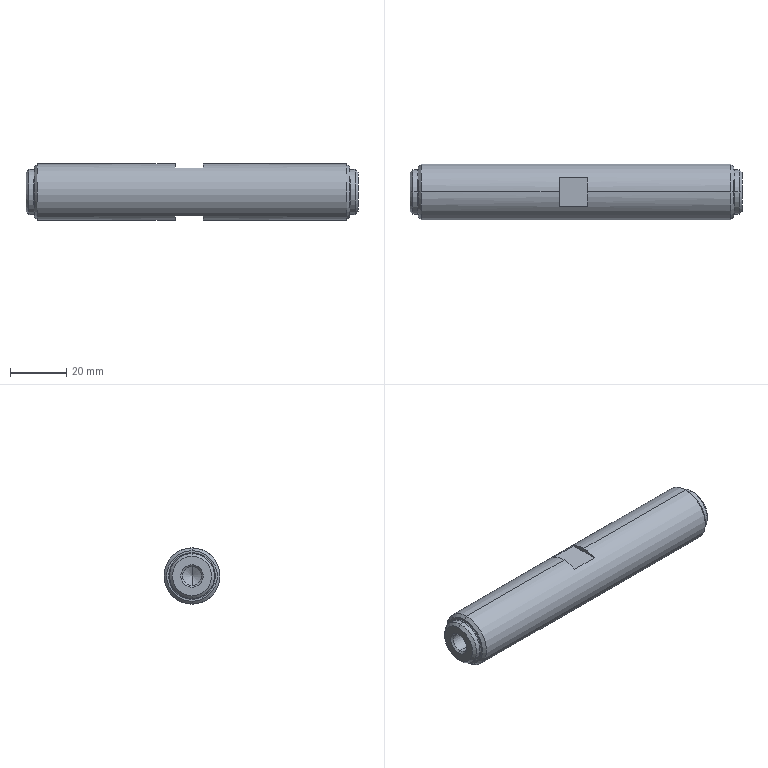Part | STEP file | sfph20_112_f3_p16_m8_t3_sc50_2_03 | 1 solid | 40 faces | box 118 x 20 x 20 mm | volume 34479 mm3 | cone 16 | cylinder 10 | plane 10 | spline 4 | commonest cylinder face diameters 6.647 x4 16 x4 20 x2